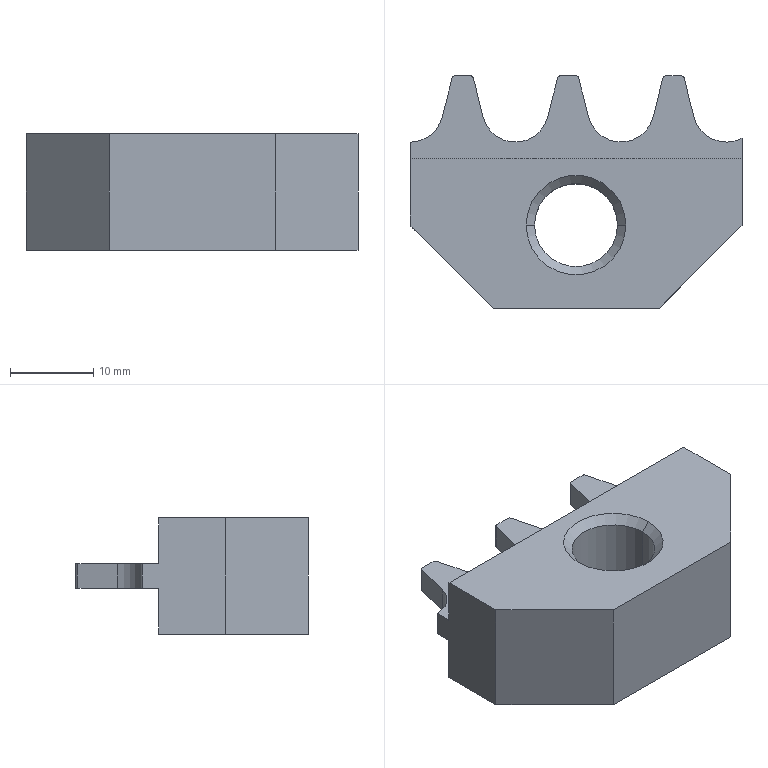Part | SolidWorks | features MirrorStock 1 | 1 solid | 36 faces | box 40 x 28 x 14 mm | volume 8141 mm3 | plane 20 | cylinder 12 | cone 4 | commonest cylinder face diameters 0.7 x6 8 x4 10 x2
STEP:
#1=CARTESIAN_POINT('',(5.,10.,-6.));
#2=VERTEX_POINT('',#1);
#3=CARTESIAN_POINT('',(-5.,10.,-6.));
#4=VERTEX_POINT('',#3);
#5=CARTESIAN_POINT('',(0.,10.,-6.));
#6=DIRECTION('',(0.,0.,1.));
#7=DIRECTION('',(-1.,0.,0.));
#8=AXIS2_PLACEMENT_3D('',#5,#6,#7);
#9=CIRCLE('',#8,5.);
#10=EDGE_CURVE('',#2,#4,#9,.T.);
#11=ORIENTED_EDGE('',*,*,#10,.T.);
#12=CARTESIAN_POINT('',(-6.,10.,-7.));
#13=VERTEX_POINT('',#12);
#14=CARTESIAN_POINT('',(-5.,10.,-6.));
#15=DIRECTION('',(-0.7071,0.,-0.7071));
#16=VECTOR('',#15,1000.);
#17=LINE('',#14,#16);
#18=EDGE_CURVE('',#4,#13,#17,.T.);
#19=ORIENTED_EDGE('',*,*,#18,.T.);
#20=CARTESIAN_POINT('',(6.,10.,-7.));
#21=VERTEX_POINT('',#20);
#22=CARTESIAN_POINT('',(0.,10.,-7.));
#23=DIRECTION('',(0.,0.,-1.));
#24=DIRECTION('',(-1.,0.,0.));
#25=AXIS2_PLACEMENT_3D('',#22,#23,#24);
#26=CIRCLE('',#25,6.);
#27=EDGE_CURVE('',#13,#21,#26,.T.);
#28=ORIENTED_EDGE('',*,*,#27,.T.);
#29=CARTESIAN_POINT('',(5.,10.,-6.));
#30=DIRECTION('',(0.7071,0.,-0.7071));
#31=VECTOR('',#30,1000.);
#32=LINE('',#29,#31);
#33=EDGE_CURVE('',#2,#21,#32,.T.);
#34=ORIENTED_EDGE('',*,*,#33,.F.);
#35=EDGE_LOOP('',(#11,#19,#28,#34));
#36=FACE_OUTER_BOUND('',#35,.T.);
#37=CARTESIAN_POINT('',(0.,10.,-6.));
#38=DIRECTION('',(0.,0.,-1.));
#39=DIRECTION('',(1.,0.,0.));
#40=AXIS2_PLACEMENT_3D('',#37,#38,#39);
#41=CONICAL_SURFACE('',#40,5.,0.7854);
#42=ADVANCED_FACE('',(#36),#41,.F.);
#43=CARTESIAN_POINT('',(-5.,10.,6.));
#44=VERTEX_POINT('',#43);
#45=CARTESIAN_POINT('',(5.,10.,6.));
#46=VERTEX_POINT('',#45);
#47=CARTESIAN_POINT('',(0.,10.,6.));
#48=DIRECTION('',(0.,0.,-1.));
#49=DIRECTION('',(-1.,0.,0.));
#50=AXIS2_PLACEMENT_3D('',#47,#48,#49);
#51=CIRCLE('',#50,5.);
#52=EDGE_CURVE('',#44,#46,#51,.T.);
#53=ORIENTED_EDGE('',*,*,#52,.T.);
#54=CARTESIAN_POINT('',(6.,10.,7.));
#55=VERTEX_POINT('',#54);
#56=CARTESIAN_POINT('',(6.,10.,7.));
#57=DIRECTION('',(0.7071,0.,0.7071));
#58=VECTOR('',#57,1000.);
#59=LINE('',#56,#58);
#60=EDGE_CURVE('',#46,#55,#59,.T.);
#61=ORIENTED_EDGE('',*,*,#60,.T.);
#62=CARTESIAN_POINT('',(-6.,10.,7.));
#63=VERTEX_POINT('',#62);
#64=CARTESIAN_POINT('',(0.,10.,7.));
#65=DIRECTION('',(0.,0.,1.));
#66=DIRECTION('',(-1.,0.,0.));
#67=AXIS2_PLACEMENT_3D('',#64,#65,#66);
#68=CIRCLE('',#67,6.);
#69=EDGE_CURVE('',#55,#63,#68,.T.);
#70=ORIENTED_EDGE('',*,*,#69,.T.);
#71=CARTESIAN_POINT('',(-6.,10.,7.));
#72=DIRECTION('',(-0.7071,0.,0.7071));
#73=VECTOR('',#72,1000.);
#74=LINE('',#71,#73);
#75=EDGE_CURVE('',#44,#63,#74,.T.);
#76=ORIENTED_EDGE('',*,*,#75,.F.);
#77=EDGE_LOOP('',(#53,#61,#70,#76));
#78=FACE_OUTER_BOUND('',#77,.T.);
#79=CARTESIAN_POINT('',(0.,10.,7.));
#80=DIRECTION('',(0.,0.,1.));
#81=DIRECTION('',(-1.,0.,0.));
#82=AXIS2_PLACEMENT_3D('',#79,#80,#81);
#83=CONICAL_SURFACE('',#82,6.,0.7854);
#84=ADVANCED_FACE('',(#78),#83,.F.);
#85=ORIENTED_EDGE('',*,*,#10,.F.);
#86=CARTESIAN_POINT('',(5.,10.,-7.));
#87=DIRECTION('',(0.,0.,1.));
#88=VECTOR('',#87,1000.);
#89=LINE('',#86,#88);
#90=EDGE_CURVE('',#2,#46,#89,.T.);
#91=ORIENTED_EDGE('',*,*,#90,.T.);
#92=ORIENTED_EDGE('',*,*,#52,.F.);
#93=CARTESIAN_POINT('',(-5.,10.,-7.));
#94=DIRECTION('',(0.,0.,1.));
#95=VECTOR('',#94,1000.);
#96=LINE('',#93,#95);
#97=EDGE_CURVE('',#4,#44,#96,.T.);
#98=ORIENTED_EDGE('',*,*,#97,.F.);
#99=EDGE_LOOP('',(#85,#91,#92,#98));
#100=FACE_OUTER_BOUND('',#99,.T.);
#101=CARTESIAN_POINT('',(0.,10.,-7.));
#102=DIRECTION('',(0.,0.,1.));
#103=DIRECTION('',(-1.,0.,0.));
#104=AXIS2_PLACEMENT_3D('',#101,#102,#103);
#105=CYLINDRICAL_SURFACE('',#104,5.);
#106=ADVANCED_FACE('',(#100),#105,.F.);
#107=CARTESIAN_POINT('',(-20.,18.,-1.5));
#108=VERTEX_POINT('',#107);
#109=CARTESIAN_POINT('',(20.,18.,-1.5));
#110=VERTEX_POINT('',#109);
#111=CARTESIAN_POINT('',(-20.,18.,-1.5));
#112=DIRECTION('',(1.,0.,0.));
#113=VECTOR('',#112,1000.);
#114=LINE('',#111,#113);
#115=EDGE_CURVE('',#108,#110,#114,.T.);
#116=ORIENTED_EDGE('',*,*,#115,.T.);
#117=CARTESIAN_POINT('',(20.,18.,-7.));
#118=VERTEX_POINT('',#117);
#119=CARTESIAN_POINT('',(20.,18.,-7.));
#120=DIRECTION('',(0.,0.,1.));
#121=VECTOR('',#120,1000.);
#122=LINE('',#119,#121);
#123=EDGE_CURVE('',#118,#110,#122,.T.);
#124=ORIENTED_EDGE('',*,*,#123,.F.);
#125=CARTESIAN_POINT('',(-20.,18.,-7.));
#126=VERTEX_POINT('',#125);
#127=CARTESIAN_POINT('',(20.,18.,-7.));
#128=DIRECTION('',(-1.,0.,0.));
#129=VECTOR('',#128,1000.);
#130=LINE('',#127,#129);
#131=EDGE_CURVE('',#118,#126,#130,.T.);
#132=ORIENTED_EDGE('',*,*,#131,.T.);
#133=CARTESIAN_POINT('',(-20.,18.,-7.));
#134=DIRECTION('',(0.,0.,1.));
#135=VECTOR('',#134,1000.);
#136=LINE('',#133,#135);
#137=EDGE_CURVE('',#126,#108,#136,.T.);
#138=ORIENTED_EDGE('',*,*,#137,.T.);
#139=EDGE_LOOP('',(#116,#124,#132,#138));
#140=FACE_OUTER_BOUND('',#139,.T.);
#141=CARTESIAN_POINT('',(20.,18.,-7.));
#142=DIRECTION('',(0.,-1.,0.));
#143=DIRECTION('',(0.,0.,1.));
#144=AXIS2_PLACEMENT_3D('',#141,#142,#143);
#145=PLANE('',#144);
#146=ADVANCED_FACE('',(#140),#145,.F.);
#147=CARTESIAN_POINT('',(0.,10.,-7.));
#148=DIRECTION('',(0.,0.,-1.));
#149=DIRECTION('',(-1.,0.,0.));
#150=AXIS2_PLACEMENT_3D('',#147,#148,#149);
#151=CIRCLE('',#150,6.);
#152=EDGE_CURVE('',#21,#13,#151,.T.);
#153=ORIENTED_EDGE('',*,*,#152,.F.);
#154=ORIENTED_EDGE('',*,*,#27,.F.);
#155=EDGE_LOOP('',(#153,#154));
#156=FACE_BOUND('',#155,.T.);
#157=CARTESIAN_POINT('',(-20.,10.,-7.));
#158=VERTEX_POINT('',#157);
#159=CARTESIAN_POINT('',(-20.,18.,-7.));
#160=DIRECTION('',(0.,-1.,0.));
#161=VECTOR('',#160,1000.);
#162=LINE('',#159,#161);
#163=EDGE_CURVE('',#126,#158,#162,.T.);
#164=ORIENTED_EDGE('',*,*,#163,.F.);
#165=ORIENTED_EDGE('',*,*,#131,.F.);
#166=CARTESIAN_POINT('',(20.,10.,-7.));
#167=VERTEX_POINT('',#166);
#168=CARTESIAN_POINT('',(20.,18.,-7.));
#169=DIRECTION('',(0.,1.,0.));
#170=VECTOR('',#169,1000.);
#171=LINE('',#168,#170);
#172=EDGE_CURVE('',#167,#118,#171,.T.);
#173=ORIENTED_EDGE('',*,*,#172,.F.);
#174=CARTESIAN_POINT('',(10.,0.,-7.));
#175=VERTEX_POINT('',#174);
#176=CARTESIAN_POINT('',(10.,0.,-7.));
#177=DIRECTION('',(0.7071,0.7071,0.));
#178=VECTOR('',#177,1000.);
#179=LINE('',#176,#178);
#180=EDGE_CURVE('',#175,#167,#179,.T.);
#181=ORIENTED_EDGE('',*,*,#180,.F.);
#182=CARTESIAN_POINT('',(-10.,0.,-7.));
#183=VERTEX_POINT('',#182);
#184=CARTESIAN_POINT('',(10.,0.,-7.));
#185=DIRECTION('',(1.,0.,0.));
#186=VECTOR('',#185,1000.);
#187=LINE('',#184,#186);
#188=EDGE_CURVE('',#183,#175,#187,.T.);
#189=ORIENTED_EDGE('',*,*,#188,.F.);
#190=CARTESIAN_POINT('',(-10.,0.,-7.));
#191=DIRECTION('',(0.7071,-0.7071,0.));
#192=VECTOR('',#191,1000.);
#193=LINE('',#190,#192);
#194=EDGE_CURVE('',#158,#183,#193,.T.);
#195=ORIENTED_EDGE('',*,*,#194,.F.);
#196=EDGE_LOOP('',(#164,#165,#173,#181,#189,#195));
#197=FACE_OUTER_BOUND('',#196,.T.);
#198=CARTESIAN_POINT('',(0.,0.,-7.));
#199=DIRECTION('',(0.,0.,1.));
#200=DIRECTION('',(-1.,0.,0.));
#201=AXIS2_PLACEMENT_3D('',#198,#199,#200);
#202=PLANE('',#201);
#203=ADVANCED_FACE('',(#156,#197),#202,.F.);
#204=CARTESIAN_POINT('',(0.,10.,7.));
#205=DIRECTION('',(0.,0.,1.));
#206=DIRECTION('',(-1.,0.,0.));
#207=AXIS2_PLACEMENT_3D('',#204,#205,#206);
#208=CIRCLE('',#207,6.);
#209=EDGE_CURVE('',#63,#55,#208,.T.);
#210=ORIENTED_EDGE('',*,*,#209,.F.);
#211=ORIENTED_EDGE('',*,*,#69,.F.);
#212=EDGE_LOOP('',(#210,#211));
#213=FACE_BOUND('',#212,.T.);
#214=CARTESIAN_POINT('',(-20.,18.,7.));
#215=VERTEX_POINT('',#214);
#216=CARTESIAN_POINT('',(-20.,10.,7.));
#217=VERTEX_POINT('',#216);
#218=CARTESIAN_POINT('',(-20.,18.,7.));
#219=DIRECTION('',(0.,-1.,0.));
#220=VECTOR('',#219,1000.);
#221=LINE('',#218,#220);
#222=EDGE_CURVE('',#215,#217,#221,.T.);
#223=ORIENTED_EDGE('',*,*,#222,.T.);
#224=CARTESIAN_POINT('',(-10.,0.,7.));
#225=VERTEX_POINT('',#224);
#226=CARTESIAN_POINT('',(-10.,0.,7.));
#227=DIRECTION('',(0.7071,-0.7071,0.));
#228=VECTOR('',#227,1000.);
#229=LINE('',#226,#228);
#230=EDGE_CURVE('',#217,#225,#229,.T.);
#231=ORIENTED_EDGE('',*,*,#230,.T.);
#232=CARTESIAN_POINT('',(10.,0.,7.));
#233=VERTEX_POINT('',#232);
#234=CARTESIAN_POINT('',(10.,0.,7.));
#235=DIRECTION('',(1.,0.,0.));
#236=VECTOR('',#235,1000.);
#237=LINE('',#234,#236);
#238=EDGE_CURVE('',#225,#233,#237,.T.);
#239=ORIENTED_EDGE('',*,*,#238,.T.);
#240=CARTESIAN_POINT('',(20.,10.,7.));
#241=VERTEX_POINT('',#240);
#242=CARTESIAN_POINT('',(10.,0.,7.));
#243=DIRECTION('',(0.7071,0.7071,0.));
#244=VECTOR('',#243,1000.);
#245=LINE('',#242,#244);
#246=EDGE_CURVE('',#233,#241,#245,.T.);
#247=ORIENTED_EDGE('',*,*,#246,.T.);
#248=CARTESIAN_POINT('',(20.,18.,7.));
#249=VERTEX_POINT('',#248);
#250=CARTESIAN_POINT('',(20.,18.,7.));
#251=DIRECTION('',(0.,1.,0.));
#252=VECTOR('',#251,1000.);
#253=LINE('',#250,#252);
#254=EDGE_CURVE('',#241,#249,#253,.T.);
#255=ORIENTED_EDGE('',*,*,#254,.T.);
#256=CARTESIAN_POINT('',(20.,18.,7.));
#257=DIRECTION('',(-1.,0.,0.));
#258=VECTOR('',#257,1000.);
#259=LINE('',#256,#258);
#260=EDGE_CURVE('',#249,#215,#259,.T.);
#261=ORIENTED_EDGE('',*,*,#260,.T.);
#262=EDGE_LOOP('',(#223,#231,#239,#247,#255,#261));
#263=FACE_OUTER_BOUND('',#262,.T.);
#264=CARTESIAN_POINT('',(0.,0.,7.));
#265=DIRECTION('',(0.,0.,1.));
#266=DIRECTION('',(-1.,0.,0.));
#267=AXIS2_PLACEMENT_3D('',#264,#265,#266);
#268=PLANE('',#267);
#269=ADVANCED_FACE('',(#213,#263),#268,.T.);
#270=ORIENTED_EDGE('',*,*,#222,.F.);
#271=CARTESIAN_POINT('',(-20.,18.,1.5));
#272=VERTEX_POINT('',#271);
#273=CARTESIAN_POINT('',(-20.,18.,-7.));
#274=DIRECTION('',(0.,0.,1.));
#275=VECTOR('',#274,1000.);
#276=LINE('',#273,#275);
#277=EDGE_CURVE('',#272,#215,#276,.T.);
#278=ORIENTED_EDGE('',*,*,#277,.F.);
#279=CARTESIAN_POINT('',(-20.,20.,1.5));
#280=VERTEX_POINT('',#279);
#281=CARTESIAN_POINT('',(-20.,18.,1.5));
#282=DIRECTION('',(0.,-1.,0.));
#283=VECTOR('',#282,1000.);
#284=LINE('',#281,#283);
#285=EDGE_CURVE('',#280,#272,#284,.T.);
#286=ORIENTED_EDGE('',*,*,#285,.F.);
#287=CARTESIAN_POINT('',(-20.,20.,-1.5));
#288=VERTEX_POINT('',#287);
#289=CARTESIAN_POINT('',(-20.,20.,-1.5));
#290=DIRECTION('',(0.,0.,1.));
#291=VECTOR('',#290,1000.);
#292=LINE('',#289,#291);
#293=EDGE_CURVE('',#288,#280,#292,.T.);
#294=ORIENTED_EDGE('',*,*,#293,.F.);
#295=CARTESIAN_POINT('',(-20.,18.,-1.5));
#296=DIRECTION('',(0.,-1.,0.));
#297=VECTOR('',#296,1000.);
#298=LINE('',#295,#297);
#299=EDGE_CURVE('',#288,#108,#298,.T.);
#300=ORIENTED_EDGE('',*,*,#299,.T.);
#301=ORIENTED_EDGE('',*,*,#137,.F.);
#302=ORIENTED_EDGE('',*,*,#163,.T.);
#303=CARTESIAN_POINT('',(-20.,10.,-7.));
#304=DIRECTION('',(0.,0.,1.));
#305=VECTOR('',#304,1000.);
#306=LINE('',#303,#305);
#307=EDGE_CURVE('',#158,#217,#306,.T.);
#308=ORIENTED_EDGE('',*,*,#307,.T.);
#309=EDGE_LOOP('',(#270,#278,#286,#294,#300,#301,#302,#308));
#310=FACE_OUTER_BOUND('',#309,.T.);
#311=CARTESIAN_POINT('',(-20.,18.,-7.));
#312=DIRECTION('',(1.,0.,0.));
#313=DIRECTION('',(0.,0.,1.));
#314=AXIS2_PLACEMENT_3D('',#311,#312,#313);
#315=PLANE('',#314);
#316=ADVANCED_FACE('',(#310),#315,.F.);
#317=ORIENTED_EDGE('',*,*,#230,.F.);
#318=ORIENTED_EDGE('',*,*,#307,.F.);
#319=ORIENTED_EDGE('',*,*,#194,.T.);
#320=CARTESIAN_POINT('',(-10.,0.,-7.));
#321=DIRECTION('',(0.,0.,1.));
#322=VECTOR('',#321,1000.);
#323=LINE('',#320,#322);
#324=EDGE_CURVE('',#183,#225,#323,.T.);
#325=ORIENTED_EDGE('',*,*,#324,.T.);
#326=EDGE_LOOP('',(#317,#318,#319,#325));
#327=FACE_OUTER_BOUND('',#326,.T.);
#328=CARTESIAN_POINT('',(-10.,0.,-7.));
#329=DIRECTION('',(0.7071,0.7071,0.));
#330=DIRECTION('',(-0.7071,0.7071,0.));
#331=AXIS2_PLACEMENT_3D('',#328,#329,#330);
#332=PLANE('',#331);
#333=ADVANCED_FACE('',(#327),#332,.F.);
#334=ORIENTED_EDGE('',*,*,#238,.F.);
#335=ORIENTED_EDGE('',*,*,#324,.F.);
#336=ORIENTED_EDGE('',*,*,#188,.T.);
#337=CARTESIAN_POINT('',(10.,0.,-7.));
#338=DIRECTION('',(0.,0.,1.));
#339=VECTOR('',#338,1000.);
#340=LINE('',#337,#339);
#341=EDGE_CURVE('',#175,#233,#340,.T.);
#342=ORIENTED_EDGE('',*,*,#341,.T.);
#343=EDGE_LOOP('',(#334,#335,#336,#342));
#344=FACE_OUTER_BOUND('',#343,.T.);
#345=CARTESIAN_POINT('',(10.,0.,-7.));
#346=DIRECTION('',(0.,1.,0.));
#347=DIRECTION('',(-1.,0.,0.));
#348=AXIS2_PLACEMENT_3D('',#345,#346,#347);
#349=PLANE('',#348);
#350=ADVANCED_FACE('',(#344),#349,.F.);
#351=ORIENTED_EDGE('',*,*,#246,.F.);
#352=ORIENTED_EDGE('',*,*,#341,.F.);
#353=ORIENTED_EDGE('',*,*,#180,.T.);
#354=CARTESIAN_POINT('',(20.,10.,-7.));
#355=DIRECTION('',(0.,0.,1.));
#356=VECTOR('',#355,1000.);
#357=LINE('',#354,#356);
#358=EDGE_CURVE('',#167,#241,#357,.T.);
#359=ORIENTED_EDGE('',*,*,#358,.T.);
#360=EDGE_LOOP('',(#351,#352,#353,#359));
#361=FACE_OUTER_BOUND('',#360,.T.);
#362=CARTESIAN_POINT('',(10.,0.,-7.));
#363=DIRECTION('',(-0.7071,0.7071,0.));
#364=DIRECTION('',(-0.7071,-0.7071,0.));
#365=AXIS2_PLACEMENT_3D('',#362,#363,#364);
#366=PLANE('',#365);
#367=ADVANCED_FACE('',(#361),#366,.F.);
#368=ORIENTED_EDGE('',*,*,#254,.F.);
#369=ORIENTED_EDGE('',*,*,#358,.F.);
#370=ORIENTED_EDGE('',*,*,#172,.T.);
#371=ORIENTED_EDGE('',*,*,#123,.T.);
#372=CARTESIAN_POINT('',(20.,20.48,-1.5));
#373=VERTEX_POINT('',#372);
#374=CARTESIAN_POINT('',(20.,18.,-1.5));
#375=DIRECTION('',(0.,1.,0.));
#376=VECTOR('',#375,1000.);
#377=LINE('',#374,#376);
#378=EDGE_CURVE('',#110,#373,#377,.T.);
#379=ORIENTED_EDGE('',*,*,#378,.T.);
#380=CARTESIAN_POINT('',(20.,20.48,1.5));
#381=VERTEX_POINT('',#380);
#382=CARTESIAN_POINT('',(20.,20.48,-1.5));
#383=DIRECTION('',(0.,0.,1.));
#384=VECTOR('',#383,1000.);
#385=LINE('',#382,#384);
#386=EDGE_CURVE('',#373,#381,#385,.T.);
#387=ORIENTED_EDGE('',*,*,#386,.T.);
#388=CARTESIAN_POINT('',(20.,18.,1.5));
#389=VERTEX_POINT('',#388);
#390=CARTESIAN_POINT('',(20.,18.,1.5));
#391=DIRECTION('',(0.,1.,0.));
#392=VECTOR('',#391,1000.);
#393=LINE('',#390,#392);
#394=EDGE_CURVE('',#389,#381,#393,.T.);
#395=ORIENTED_EDGE('',*,*,#394,.F.);
#396=CARTESIAN_POINT('',(20.,18.,-7.));
#397=DIRECTION('',(0.,0.,1.));
#398=VECTOR('',#397,1000.);
#399=LINE('',#396,#398);
#400=EDGE_CURVE('',#389,#249,#399,.T.);
#401=ORIENTED_EDGE('',*,*,#400,.T.);
#402=EDGE_LOOP('',(#368,#369,#370,#371,#379,#387,#395,#401));
#403=FACE_OUTER_BOUND('',#402,.T.);
#404=CARTESIAN_POINT('',(20.,18.,-7.));
#405=DIRECTION('',(-1.,0.,0.));
#406=DIRECTION('',(0.,0.,-1.));
#407=AXIS2_PLACEMENT_3D('',#404,#405,#406);
#408=PLANE('',#407);
#409=ADVANCED_FACE('',(#403),#408,.F.);
#410=ORIENTED_EDGE('',*,*,#277,.T.);
#411=ORIENTED_EDGE('',*,*,#260,.F.);
#412=ORIENTED_EDGE('',*,*,#400,.F.);
#413=CARTESIAN_POINT('',(-20.,18.,1.5));
#414=DIRECTION('',(1.,0.,0.));
#415=VECTOR('',#414,1000.);
#416=LINE('',#413,#415);
#417=EDGE_CURVE('',#272,#389,#416,.T.);
#418=ORIENTED_EDGE('',*,*,#417,.F.);
#419=EDGE_LOOP('',(#410,#411,#412,#418));
#420=FACE_OUTER_BOUND('',#419,.T.);
#421=CARTESIAN_POINT('',(20.,18.,-7.));
#422=DIRECTION('',(0.,-1.,0.));
#423=DIRECTION('',(0.,0.,1.));
#424=AXIS2_PLACEMENT_3D('',#421,#422,#423);
#425=PLANE('',#424);
#426=ADVANCED_FACE('',(#420),#425,.F.);
#427=ORIENTED_EDGE('',*,*,#90,.F.);
#428=CARTESIAN_POINT('',(0.,10.,-6.));
#429=DIRECTION('',(0.,0.,1.));
#430=DIRECTION('',(-1.,0.,0.));
#431=AXIS2_PLACEMENT_3D('',#428,#429,#430);
#432=CIRCLE('',#431,5.);
#433=EDGE_CURVE('',#4,#2,#432,.T.);
#434=ORIENTED_EDGE('',*,*,#433,.F.);
#435=ORIENTED_EDGE('',*,*,#97,.T.);
#436=CARTESIAN_POINT('',(0.,10.,6.));
#437=DIRECTION('',(0.,0.,-1.));
#438=DIRECTION('',(-1.,0.,0.));
#439=AXIS2_PLACEMENT_3D('',#436,#437,#438);
#440=CIRCLE('',#439,5.);
#441=EDGE_CURVE('',#46,#44,#440,.T.);
#442=ORIENTED_EDGE('',*,*,#441,.F.);
#443=EDGE_LOOP('',(#427,#434,#435,#442));
#444=FACE_OUTER_BOUND('',#443,.T.);
#445=CARTESIAN_POINT('',(0.,10.,-7.));
#446=DIRECTION('',(0.,0.,1.));
#447=DIRECTION('',(-1.,0.,0.));
#448=AXIS2_PLACEMENT_3D('',#445,#446,#447);
#449=CYLINDRICAL_SURFACE('',#448,5.);
#450=ADVANCED_FACE('',(#444),#449,.F.);
#451=CARTESIAN_POINT('',(14.224,23.01,1.5));
#452=VERTEX_POINT('',#451);
#453=CARTESIAN_POINT('',(18.1,24.,1.5));
#454=DIRECTION('',(0.,0.,-1.));
#455=DIRECTION('',(1.,0.,0.));
#456=AXIS2_PLACEMENT_3D('',#453,#454,#455);
#457=CIRCLE('',#456,4.);
#458=EDGE_CURVE('',#381,#452,#457,.T.);
#459=ORIENTED_EDGE('',*,*,#458,.F.);
#460=ORIENTED_EDGE('',*,*,#386,.F.);
#461=CARTESIAN_POINT('',(14.224,23.01,-1.5));
#462=VERTEX_POINT('',#461);
#463=CARTESIAN_POINT('',(18.1,24.,-1.5));
#464=DIRECTION('',(0.,0.,-1.));
#465=DIRECTION('',(1.,0.,0.));
#466=AXIS2_PLACEMENT_3D('',#463,#464,#465);
#467=CIRCLE('',#466,4.);
#468=EDGE_CURVE('',#373,#462,#467,.T.);
#469=ORIENTED_EDGE('',*,*,#468,.T.);
#470=CARTESIAN_POINT('',(14.224,23.01,-1.5));
#471=DIRECTION('',(0.,0.,1.));
#472=VECTOR('',#471,1000.);
#473=LINE('',#470,#472);
#474=EDGE_CURVE('',#462,#452,#473,.T.);
#475=ORIENTED_EDGE('',*,*,#474,.T.);
#476=EDGE_LOOP('',(#459,#460,#469,#475));
#477=FACE_OUTER_BOUND('',#476,.T.);
#478=CARTESIAN_POINT('',(18.1,24.,-1.5));
#479=DIRECTION('',(0.,0.,1.));
#480=DIRECTION('',(-1.,0.,0.));
#481=AXIS2_PLACEMENT_3D('',#478,#479,#480);
#482=CYLINDRICAL_SURFACE('',#481,4.);
#483=ADVANCED_FACE('',(#477),#482,.F.);
#484=CARTESIAN_POINT('',(13.017,27.737,1.5));
#485=VERTEX_POINT('',#484);
#486=CARTESIAN_POINT('',(12.95,28.,1.5));
#487=DIRECTION('',(-0.2475,0.9689,0.));
#488=VECTOR('',#487,1000.);
#489=LINE('',#486,#488);
#490=EDGE_CURVE('',#452,#485,#489,.T.);
#491=ORIENTED_EDGE('',*,*,#490,.F.);
#492=ORIENTED_EDGE('',*,*,#474,.F.);
#493=CARTESIAN_POINT('',(13.017,27.737,-1.5));
#494=VERTEX_POINT('',#493);
#495=CARTESIAN_POINT('',(12.95,28.,-1.5));
#496=DIRECTION('',(-0.2475,0.9689,0.));
#497=VECTOR('',#496,1000.);
#498=LINE('',#495,#497);
#499=EDGE_CURVE('',#462,#494,#498,.T.);
#500=ORIENTED_EDGE('',*,*,#499,.T.);
#501=CARTESIAN_POINT('',(13.017,27.737,-1.5));
#502=DIRECTION('',(0.,0.,-1.));
#503=VECTOR('',#502,1000.);
#504=LINE('',#501,#503);
#505=EDGE_CURVE('',#485,#494,#504,.T.);
#506=ORIENTED_EDGE('',*,*,#505,.F.);
#507=EDGE_LOOP('',(#491,#492,#500,#506));
#508=FACE_OUTER_BOUND('',#507,.T.);
#509=CARTESIAN_POINT('',(12.95,28.,-1.5));
#510=DIRECTION('',(-0.9689,-0.2475,0.));
#511=DIRECTION('',(0.2475,-0.9689,0.));
#512=AXIS2_PLACEMENT_3D('',#509,#510,#511);
#513=PLANE('',#512);
#514=ADVANCED_FACE('',(#508),#513,.F.);
#515=CARTESIAN_POINT('',(12.678,28.,-1.5));
#516=VERTEX_POINT('',#515);
#517=CARTESIAN_POINT('',(10.822,28.,-1.5));
#518=VERTEX_POINT('',#517);
#519=CARTESIAN_POINT('',(10.55,28.,-1.5));
#520=DIRECTION('',(-1.,0.,0.));
#521=VECTOR('',#520,1000.);
#522=LINE('',#519,#521);
#523=EDGE_CURVE('',#516,#518,#522,.T.);
#524=ORIENTED_EDGE('',*,*,#523,.T.);
#525=CARTESIAN_POINT('',(10.822,28.,1.5));
#526=VERTEX_POINT('',#525);
#527=CARTESIAN_POINT('',(10.822,28.,-1.5));
#528=DIRECTION('',(0.,0.,-1.));
#529=VECTOR('',#528,1000.);
#530=LINE('',#527,#529);
#531=EDGE_CURVE('',#526,#518,#530,.T.);
#532=ORIENTED_EDGE('',*,*,#531,.F.);
#533=CARTESIAN_POINT('',(12.678,28.,1.5));
#534=VERTEX_POINT('',#533);
#535=CARTESIAN_POINT('',(10.55,28.,1.5));
#536=DIRECTION('',(-1.,0.,0.));
#537=VECTOR('',#536,1000.);
#538=LINE('',#535,#537);
#539=EDGE_CURVE('',#534,#526,#538,.T.);
#540=ORIENTED_EDGE('',*,*,#539,.F.);
#541=CARTESIAN_POINT('',(12.678,28.,-1.5));
#542=DIRECTION('',(0.,0.,1.));
#543=VECTOR('',#542,1000.);
#544=LINE('',#541,#543);
#545=EDGE_CURVE('',#516,#534,#544,.T.);
#546=ORIENTED_EDGE('',*,*,#545,.F.);
#547=EDGE_LOOP('',(#524,#532,#540,#546));
#548=FACE_OUTER_BOUND('',#547,.T.);
#549=CARTESIAN_POINT('',(10.55,28.,-1.5));
#550=DIRECTION('',(0.,-1.,0.));
#551=DIRECTION('',(0.,0.,1.));
#552=AXIS2_PLACEMENT_3D('',#549,#550,#551);
#553=PLANE('',#552);
#554=ADVANCED_FACE('',(#548),#553,.F.);
#555=CARTESIAN_POINT('',(10.483,27.737,-1.5));
#556=VERTEX_POINT('',#555);
#557=CARTESIAN_POINT('',(9.276,23.01,-1.5));
#558=VERTEX_POINT('',#557);
#559=CARTESIAN_POINT('',(10.55,28.,-1.5));
#560=DIRECTION('',(-0.2475,-0.9689,0.));
#561=VECTOR('',#560,1000.);
#562=LINE('',#559,#561);
#563=EDGE_CURVE('',#556,#558,#562,.T.);
#564=ORIENTED_EDGE('',*,*,#563,.T.);
#565=CARTESIAN_POINT('',(9.276,23.01,1.5));
#566=VERTEX_POINT('',#565);
#567=CARTESIAN_POINT('',(9.276,23.01,-1.5));
#568=DIRECTION('',(0.,0.,1.));
#569=VECTOR('',#568,1000.);
#570=LINE('',#567,#569);
#571=EDGE_CURVE('',#558,#566,#570,.T.);
#572=ORIENTED_EDGE('',*,*,#571,.T.);
#573=CARTESIAN_POINT('',(10.483,27.737,1.5));
#574=VERTEX_POINT('',#573);
#575=CARTESIAN_POINT('',(10.55,28.,1.5));
#576=DIRECTION('',(-0.2475,-0.9689,0.));
#577=VECTOR('',#576,1000.);
#578=LINE('',#575,#577);
#579=EDGE_CURVE('',#574,#566,#578,.T.);
#580=ORIENTED_EDGE('',*,*,#579,.F.);
#581=CARTESIAN_POINT('',(10.483,27.737,-1.5));
#582=DIRECTION('',(0.,0.,1.));
#583=VECTOR('',#582,1000.);
#584=LINE('',#581,#583);
#585=EDGE_CURVE('',#556,#574,#584,.T.);
#586=ORIENTED_EDGE('',*,*,#585,.F.);
#587=EDGE_LOOP('',(#564,#572,#580,#586));
#588=FACE_OUTER_BOUND('',#587,.T.);
#589=CARTESIAN_POINT('',(10.55,28.,-1.5));
#590=DIRECTION('',(0.9689,-0.2475,0.));
#591=DIRECTION('',(0.2475,0.9689,0.));
#592=AXIS2_PLACEMENT_3D('',#589,#590,#591);
#593=PLANE('',#592);
#594=ADVANCED_FACE('',(#588),#593,.F.);
#595=CARTESIAN_POINT('',(1.524,23.01,1.5));
#596=VERTEX_POINT('',#595);
#597=CARTESIAN_POINT('',(5.4,24.,1.5));
#598=DIRECTION('',(0.,0.,-1.));
#599=DIRECTION('',(1.,0.,0.));
#600=AXIS2_PLACEMENT_3D('',#597,#598,#599);
#601=CIRCLE('',#600,4.);
#602=EDGE_CURVE('',#566,#596,#601,.T.);
#603=ORIENTED_EDGE('',*,*,#602,.F.);
#604=ORIENTED_EDGE('',*,*,#571,.F.);
#605=CARTESIAN_POINT('',(1.524,23.01,-1.5));
#606=VERTEX_POINT('',#605);
#607=CARTESIAN_POINT('',(5.4,24.,-1.5));
#608=DIRECTION('',(0.,0.,-1.));
#609=DIRECTION('',(1.,0.,0.));
#610=AXIS2_PLACEMENT_3D('',#607,#608,#609);
#611=CIRCLE('',#610,4.);
#612=EDGE_CURVE('',#558,#606,#611,.T.);
#613=ORIENTED_EDGE('',*,*,#612,.T.);
#614=CARTESIAN_POINT('',(1.524,23.01,-1.5));
#615=DIRECTION('',(0.,0.,1.));
#616=VECTOR('',#615,1000.);
#617=LINE('',#614,#616);
#618=EDGE_CURVE('',#606,#596,#617,.T.);
#619=ORIENTED_EDGE('',*,*,#618,.T.);
#620=EDGE_LOOP('',(#603,#604,#613,#619));
#621=FACE_OUTER_BOUND('',#620,.T.);
#622=CARTESIAN_POINT('',(5.4,24.,-1.5));
#623=DIRECTION('',(0.,0.,1.));
#624=DIRECTION('',(-1.,0.,0.));
#625=AXIS2_PLACEMENT_3D('',#622,#623,#624);
#626=CYLINDRICAL_SURFACE('',#625,4.);
#627=ADVANCED_FACE('',(#621),#626,.F.);
#628=CARTESIAN_POINT('',(0.3173,27.737,1.5));
#629=VERTEX_POINT('',#628);
#630=CARTESIAN_POINT('',(0.25,28.,1.5));
#631=DIRECTION('',(-0.2475,0.9689,0.));
#632=VECTOR('',#631,1000.);
#633=LINE('',#630,#632);
#634=EDGE_CURVE('',#596,#629,#633,.T.);
#635=ORIENTED_EDGE('',*,*,#634,.F.);
#636=ORIENTED_EDGE('',*,*,#618,.F.);
#637=CARTESIAN_POINT('',(0.3173,27.737,-1.5));
#638=VERTEX_POINT('',#637);
#639=CARTESIAN_POINT('',(0.25,28.,-1.5));
#640=DIRECTION('',(-0.2475,0.9689,0.));
#641=VECTOR('',#640,1000.);
#642=LINE('',#639,#641);
#643=EDGE_CURVE('',#606,#638,#642,.T.);
#644=ORIENTED_EDGE('',*,*,#643,.T.);
#645=CARTESIAN_POINT('',(0.3173,27.737,-1.5));
#646=DIRECTION('',(0.,0.,-1.));
#647=VECTOR('',#646,1000.);
#648=LINE('',#645,#647);
#649=EDGE_CURVE('',#629,#638,#648,.T.);
#650=ORIENTED_EDGE('',*,*,#649,.F.);
#651=EDGE_LOOP('',(#635,#636,#644,#650));
#652=FACE_OUTER_BOUND('',#651,.T.);
#653=CARTESIAN_POINT('',(0.25,28.,-1.5));
#654=DIRECTION('',(-0.9689,-0.2475,0.));
#655=DIRECTION('',(0.2475,-0.9689,0.));
#656=AXIS2_PLACEMENT_3D('',#653,#654,#655);
#657=PLANE('',#656);
#658=ADVANCED_FACE('',(#652),#657,.F.);
#659=CARTESIAN_POINT('',(-0.02184,28.,-1.5));
#660=VERTEX_POINT('',#659);
#661=CARTESIAN_POINT('',(-1.878,28.,-1.5));
#662=VERTEX_POINT('',#661);
#663=CARTESIAN_POINT('',(-2.15,28.,-1.5));
#664=DIRECTION('',(-1.,0.,0.));
#665=VECTOR('',#664,1000.);
#666=LINE('',#663,#665);
#667=EDGE_CURVE('',#660,#662,#666,.T.);
#668=ORIENTED_EDGE('',*,*,#667,.T.);
#669=CARTESIAN_POINT('',(-1.878,28.,1.5));
#670=VERTEX_POINT('',#669);
#671=CARTESIAN_POINT('',(-1.878,28.,-1.5));
#672=DIRECTION('',(0.,0.,-1.));
#673=VECTOR('',#672,1000.);
#674=LINE('',#671,#673);
#675=EDGE_CURVE('',#670,#662,#674,.T.);
#676=ORIENTED_EDGE('',*,*,#675,.F.);
#677=CARTESIAN_POINT('',(-0.02184,28.,1.5));
#678=VERTEX_POINT('',#677);
#679=CARTESIAN_POINT('',(-2.15,28.,1.5));
#680=DIRECTION('',(-1.,0.,0.));
#681=VECTOR('',#680,1000.);
#682=LINE('',#679,#681);
#683=EDGE_CURVE('',#678,#670,#682,.T.);
#684=ORIENTED_EDGE('',*,*,#683,.F.);
#685=CARTESIAN_POINT('',(-0.02184,28.,-1.5));
#686=DIRECTION('',(0.,0.,1.));
#687=VECTOR('',#686,1000.);
#688=LINE('',#685,#687);
#689=EDGE_CURVE('',#660,#678,#688,.T.);
#690=ORIENTED_EDGE('',*,*,#689,.F.);
#691=EDGE_LOOP('',(#668,#676,#684,#690));
#692=FACE_OUTER_BOUND('',#691,.T.);
#693=CARTESIAN_POINT('',(-2.15,28.,-1.5));
#694=DIRECTION('',(0.,-1.,0.));
#695=DIRECTION('',(0.,0.,1.));
#696=AXIS2_PLACEMENT_3D('',#693,#694,#695);
#697=PLANE('',#696);
#698=ADVANCED_FACE('',(#692),#697,.F.);
#699=CARTESIAN_POINT('',(-2.217,27.737,-1.5));
#700=VERTEX_POINT('',#699);
#701=CARTESIAN_POINT('',(-3.424,23.01,-1.5));
#702=VERTEX_POINT('',#701);
#703=CARTESIAN_POINT('',(-2.15,28.,-1.5));
#704=DIRECTION('',(-0.2475,-0.9689,0.));
#705=VECTOR('',#704,1000.);
#706=LINE('',#703,#705);
#707=EDGE_CURVE('',#700,#702,#706,.T.);
#708=ORIENTED_EDGE('',*,*,#707,.T.);
#709=CARTESIAN_POINT('',(-3.424,23.01,1.5));
#710=VERTEX_POINT('',#709);
#711=CARTESIAN_POINT('',(-3.424,23.01,-1.5));
#712=DIRECTION('',(0.,0.,1.));
#713=VECTOR('',#712,1000.);
#714=LINE('',#711,#713);
#715=EDGE_CURVE('',#702,#710,#714,.T.);
#716=ORIENTED_EDGE('',*,*,#715,.T.);
#717=CARTESIAN_POINT('',(-2.217,27.737,1.5));
#718=VERTEX_POINT('',#717);
#719=CARTESIAN_POINT('',(-2.15,28.,1.5));
#720=DIRECTION('',(-0.2475,-0.9689,0.));
#721=VECTOR('',#720,1000.);
#722=LINE('',#719,#721);
#723=EDGE_CURVE('',#718,#710,#722,.T.);
#724=ORIENTED_EDGE('',*,*,#723,.F.);
#725=CARTESIAN_POINT('',(-2.217,27.737,-1.5));
#726=DIRECTION('',(0.,0.,1.));
#727=VECTOR('',#726,1000.);
#728=LINE('',#725,#727);
#729=EDGE_CURVE('',#700,#718,#728,.T.);
#730=ORIENTED_EDGE('',*,*,#729,.F.);
#731=EDGE_LOOP('',(#708,#716,#724,#730));
#732=FACE_OUTER_BOUND('',#731,.T.);
#733=CARTESIAN_POINT('',(-2.15,28.,-1.5));
#734=DIRECTION('',(0.9689,-0.2475,0.));
#735=DIRECTION('',(0.2475,0.9689,0.));
#736=AXIS2_PLACEMENT_3D('',#733,#734,#735);
#737=PLANE('',#736);
#738=ADVANCED_FACE('',(#732),#737,.F.);
#739=CARTESIAN_POINT('',(-11.176,23.01,1.5));
#740=VERTEX_POINT('',#739);
#741=CARTESIAN_POINT('',(-7.3,24.,1.5));
#742=DIRECTION('',(0.,0.,-1.));
#743=DIRECTION('',(1.,0.,0.));
#744=AXIS2_PLACEMENT_3D('',#741,#742,#743);
#745=CIRCLE('',#744,4.);
#746=EDGE_CURVE('',#710,#740,#745,.T.);
#747=ORIENTED_EDGE('',*,*,#746,.F.);
#748=ORIENTED_EDGE('',*,*,#715,.F.);
#749=CARTESIAN_POINT('',(-11.176,23.01,-1.5));
#750=VERTEX_POINT('',#749);
#751=CARTESIAN_POINT('',(-7.3,24.,-1.5));
#752=DIRECTION('',(0.,0.,-1.));
#753=DIRECTION('',(1.,0.,0.));
#754=AXIS2_PLACEMENT_3D('',#751,#752,#753);
#755=CIRCLE('',#754,4.);
#756=EDGE_CURVE('',#702,#750,#755,.T.);
#757=ORIENTED_EDGE('',*,*,#756,.T.);
#758=CARTESIAN_POINT('',(-11.176,23.01,-1.5));
#759=DIRECTION('',(0.,0.,1.));
#760=VECTOR('',#759,1000.);
#761=LINE('',#758,#760);
#762=EDGE_CURVE('',#750,#740,#761,.T.);
#763=ORIENTED_EDGE('',*,*,#762,.T.);
#764=EDGE_LOOP('',(#747,#748,#757,#763));
#765=FACE_OUTER_BOUND('',#764,.T.);
#766=CARTESIAN_POINT('',(-7.3,24.,-1.5));
#767=DIRECTION('',(0.,0.,1.));
#768=DIRECTION('',(-1.,0.,0.));
#769=AXIS2_PLACEMENT_3D('',#766,#767,#768);
#770=CYLINDRICAL_SURFACE('',#769,4.);
#771=ADVANCED_FACE('',(#765),#770,.F.);
#772=CARTESIAN_POINT('',(-12.383,27.737,1.5));
#773=VERTEX_POINT('',#772);
#774=CARTESIAN_POINT('',(-12.45,28.,1.5));
#775=DIRECTION('',(-0.2475,0.9689,0.));
#776=VECTOR('',#775,1000.);
#777=LINE('',#774,#776);
#778=EDGE_CURVE('',#740,#773,#777,.T.);
#779=ORIENTED_EDGE('',*,*,#778,.F.);
#780=ORIENTED_EDGE('',*,*,#762,.F.);
#781=CARTESIAN_POINT('',(-12.383,27.737,-1.5));
#782=VERTEX_POINT('',#781);
#783=CARTESIAN_POINT('',(-12.45,28.,-1.5));
#784=DIRECTION('',(-0.2475,0.9689,0.));
#785=VECTOR('',#784,1000.);
#786=LINE('',#783,#785);
#787=EDGE_CURVE('',#750,#782,#786,.T.);
#788=ORIENTED_EDGE('',*,*,#787,.T.);
#789=CARTESIAN_POINT('',(-12.383,27.737,-1.5));
#790=DIRECTION('',(0.,0.,-1.));
#791=VECTOR('',#790,1000.);
#792=LINE('',#789,#791);
#793=EDGE_CURVE('',#773,#782,#792,.T.);
#794=ORIENTED_EDGE('',*,*,#793,.F.);
#795=EDGE_LOOP('',(#779,#780,#788,#794));
#796=FACE_OUTER_BOUND('',#795,.T.);
#797=CARTESIAN_POINT('',(-12.45,28.,-1.5));
#798=DIRECTION('',(-0.9689,-0.2475,0.));
#799=DIRECTION('',(0.2475,-0.9689,0.));
#800=AXIS2_PLACEMENT_3D('',#797,#798,#799);
#801=PLANE('',#800);
#802=ADVANCED_FACE('',(#796),#801,.F.);
#803=CARTESIAN_POINT('',(-12.722,28.,-1.5));
#804=VERTEX_POINT('',#803);
#805=CARTESIAN_POINT('',(-14.578,28.,-1.5));
#806=VERTEX_POINT('',#805);
#807=CARTESIAN_POINT('',(-14.85,28.,-1.5));
#808=DIRECTION('',(-1.,0.,0.));
#809=VECTOR('',#808,1000.);
#810=LINE('',#807,#809);
#811=EDGE_CURVE('',#804,#806,#810,.T.);
#812=ORIENTED_EDGE('',*,*,#811,.T.);
#813=CARTESIAN_POINT('',(-14.578,28.,1.5));
#814=VERTEX_POINT('',#813);
#815=CARTESIAN_POINT('',(-14.578,28.,-1.5));
#816=DIRECTION('',(0.,0.,-1.));
#817=VECTOR('',#816,1000.);
#818=LINE('',#815,#817);
#819=EDGE_CURVE('',#814,#806,#818,.T.);
#820=ORIENTED_EDGE('',*,*,#819,.F.);
#821=CARTESIAN_POINT('',(-12.722,28.,1.5));
#822=VERTEX_POINT('',#821);
#823=CARTESIAN_POINT('',(-14.85,28.,1.5));
#824=DIRECTION('',(-1.,0.,0.));
#825=VECTOR('',#824,1000.);
#826=LINE('',#823,#825);
#827=EDGE_CURVE('',#822,#814,#826,.T.);
#828=ORIENTED_EDGE('',*,*,#827,.F.);
#829=CARTESIAN_POINT('',(-12.722,28.,-1.5));
#830=DIRECTION('',(0.,0.,1.));
#831=VECTOR('',#830,1000.);
#832=LINE('',#829,#831);
#833=EDGE_CURVE('',#804,#822,#832,.T.);
#834=ORIENTED_EDGE('',*,*,#833,.F.);
#835=EDGE_LOOP('',(#812,#820,#828,#834));
#836=FACE_OUTER_BOUND('',#835,.T.);
#837=CARTESIAN_POINT('',(-14.85,28.,-1.5));
#838=DIRECTION('',(0.,-1.,0.));
#839=DIRECTION('',(0.,0.,1.));
#840=AXIS2_PLACEMENT_3D('',#837,#838,#839);
#841=PLANE('',#840);
#842=ADVANCED_FACE('',(#836),#841,.F.);
#843=CARTESIAN_POINT('',(-14.917,27.737,-1.5));
#844=VERTEX_POINT('',#843);
#845=CARTESIAN_POINT('',(-16.124,23.01,-1.5));
#846=VERTEX_POINT('',#845);
#847=CARTESIAN_POINT('',(-14.85,28.,-1.5));
#848=DIRECTION('',(-0.2475,-0.9689,0.));
#849=VECTOR('',#848,1000.);
#850=LINE('',#847,#849);
#851=EDGE_CURVE('',#844,#846,#850,.T.);
#852=ORIENTED_EDGE('',*,*,#851,.T.);
#853=CARTESIAN_POINT('',(-16.124,23.01,1.5));
#854=VERTEX_POINT('',#853);
#855=CARTESIAN_POINT('',(-16.124,23.01,-1.5));
#856=DIRECTION('',(0.,0.,1.));
#857=VECTOR('',#856,1000.);
#858=LINE('',#855,#857);
#859=EDGE_CURVE('',#846,#854,#858,.T.);
#860=ORIENTED_EDGE('',*,*,#859,.T.);
#861=CARTESIAN_POINT('',(-14.917,27.737,1.5));
#862=VERTEX_POINT('',#861);
#863=CARTESIAN_POINT('',(-14.85,28.,1.5));
#864=DIRECTION('',(-0.2475,-0.9689,0.));
#865=VECTOR('',#864,1000.);
#866=LINE('',#863,#865);
#867=EDGE_CURVE('',#862,#854,#866,.T.);
#868=ORIENTED_EDGE('',*,*,#867,.F.);
#869=CARTESIAN_POINT('',(-14.917,27.737,-1.5));
#870=DIRECTION('',(0.,0.,1.));
#871=VECTOR('',#870,1000.);
#872=LINE('',#869,#871);
#873=EDGE_CURVE('',#844,#862,#872,.T.);
#874=ORIENTED_EDGE('',*,*,#873,.F.);
#875=EDGE_LOOP('',(#852,#860,#868,#874));
#876=FACE_OUTER_BOUND('',#875,.T.);
#877=CARTESIAN_POINT('',(-14.85,28.,-1.5));
#878=DIRECTION('',(0.9689,-0.2475,0.));
#879=DIRECTION('',(0.2475,0.9689,0.));
#880=AXIS2_PLACEMENT_3D('',#877,#878,#879);
#881=PLANE('',#880);
#882=ADVANCED_FACE('',(#876),#881,.F.);
#883=CARTESIAN_POINT('',(-20.,24.,1.5));
#884=DIRECTION('',(0.,0.,-1.));
#885=DIRECTION('',(1.,0.,0.));
#886=AXIS2_PLACEMENT_3D('',#883,#884,#885);
#887=CIRCLE('',#886,4.);
#888=EDGE_CURVE('',#854,#280,#887,.T.);
#889=ORIENTED_EDGE('',*,*,#888,.F.);
#890=ORIENTED_EDGE('',*,*,#859,.F.);
#891=CARTESIAN_POINT('',(-20.,24.,-1.5));
#892=DIRECTION('',(0.,0.,-1.));
#893=DIRECTION('',(1.,0.,0.));
#894=AXIS2_PLACEMENT_3D('',#891,#892,#893);
#895=CIRCLE('',#894,4.);
#896=EDGE_CURVE('',#846,#288,#895,.T.);
#897=ORIENTED_EDGE('',*,*,#896,.T.);
#898=ORIENTED_EDGE('',*,*,#293,.T.);
#899=EDGE_LOOP('',(#889,#890,#897,#898));
#900=FACE_OUTER_BOUND('',#899,.T.);
#901=CARTESIAN_POINT('',(-20.,24.,-1.5));
#902=DIRECTION('',(0.,0.,1.));
#903=DIRECTION('',(-1.,0.,0.));
#904=AXIS2_PLACEMENT_3D('',#901,#902,#903);
#905=CYLINDRICAL_SURFACE('',#904,4.);
#906=ADVANCED_FACE('',(#900),#905,.F.);
#907=ORIENTED_EDGE('',*,*,#499,.F.);
#908=ORIENTED_EDGE('',*,*,#468,.F.);
#909=ORIENTED_EDGE('',*,*,#378,.F.);
#910=ORIENTED_EDGE('',*,*,#115,.F.);
#911=ORIENTED_EDGE('',*,*,#299,.F.);
#912=ORIENTED_EDGE('',*,*,#896,.F.);
#913=ORIENTED_EDGE('',*,*,#851,.F.);
#914=CARTESIAN_POINT('',(-14.578,27.65,-1.5));
#915=DIRECTION('',(0.,0.,1.));
#916=DIRECTION('',(1.,0.,0.));
#917=AXIS2_PLACEMENT_3D('',#914,#915,#916);
#918=CIRCLE('',#917,0.35);
#919=EDGE_CURVE('',#806,#844,#918,.T.);
#920=ORIENTED_EDGE('',*,*,#919,.F.);
#921=ORIENTED_EDGE('',*,*,#811,.F.);
#922=CARTESIAN_POINT('',(-12.722,27.65,-1.5));
#923=DIRECTION('',(0.,0.,1.));
#924=DIRECTION('',(1.,0.,0.));
#925=AXIS2_PLACEMENT_3D('',#922,#923,#924);
#926=CIRCLE('',#925,0.35);
#927=EDGE_CURVE('',#782,#804,#926,.T.);
#928=ORIENTED_EDGE('',*,*,#927,.F.);
#929=ORIENTED_EDGE('',*,*,#787,.F.);
#930=ORIENTED_EDGE('',*,*,#756,.F.);
#931=ORIENTED_EDGE('',*,*,#707,.F.);
#932=CARTESIAN_POINT('',(-1.878,27.65,-1.5));
#933=DIRECTION('',(0.,0.,1.));
#934=DIRECTION('',(1.,0.,0.));
#935=AXIS2_PLACEMENT_3D('',#932,#933,#934);
#936=CIRCLE('',#935,0.35);
#937=EDGE_CURVE('',#662,#700,#936,.T.);
#938=ORIENTED_EDGE('',*,*,#937,.F.);
#939=ORIENTED_EDGE('',*,*,#667,.F.);
#940=CARTESIAN_POINT('',(-0.02184,27.65,-1.5));
#941=DIRECTION('',(0.,0.,1.));
#942=DIRECTION('',(1.,0.,0.));
#943=AXIS2_PLACEMENT_3D('',#940,#941,#942);
#944=CIRCLE('',#943,0.35);
#945=EDGE_CURVE('',#638,#660,#944,.T.);
#946=ORIENTED_EDGE('',*,*,#945,.F.);
#947=ORIENTED_EDGE('',*,*,#643,.F.);
#948=ORIENTED_EDGE('',*,*,#612,.F.);
#949=ORIENTED_EDGE('',*,*,#563,.F.);
#950=CARTESIAN_POINT('',(10.822,27.65,-1.5));
#951=DIRECTION('',(0.,0.,1.));
#952=DIRECTION('',(1.,0.,0.));
#953=AXIS2_PLACEMENT_3D('',#950,#951,#952);
#954=CIRCLE('',#953,0.35);
#955=EDGE_CURVE('',#518,#556,#954,.T.);
#956=ORIENTED_EDGE('',*,*,#955,.F.);
#957=ORIENTED_EDGE('',*,*,#523,.F.);
#958=CARTESIAN_POINT('',(12.678,27.65,-1.5));
#959=DIRECTION('',(0.,0.,1.));
#960=DIRECTION('',(1.,0.,0.));
#961=AXIS2_PLACEMENT_3D('',#958,#959,#960);
#962=CIRCLE('',#961,0.35);
#963=EDGE_CURVE('',#494,#516,#962,.T.);
#964=ORIENTED_EDGE('',*,*,#963,.F.);
#965=EDGE_LOOP('',(#907,#908,#909,#910,#911,#912,#913,#920,#921,#928,#929,#930,#931,#938,#939,#946,#947,#948,#949,#956,#957,#964));
#966=FACE_OUTER_BOUND('',#965,.T.);
#967=CARTESIAN_POINT('',(18.1,24.,-1.5));
#968=DIRECTION('',(0.,0.,-1.));
#969=DIRECTION('',(1.,0.,0.));
#970=AXIS2_PLACEMENT_3D('',#967,#968,#969);
#971=PLANE('',#970);
#972=ADVANCED_FACE('',(#966),#971,.T.);
#973=ORIENTED_EDGE('',*,*,#539,.T.);
#974=CARTESIAN_POINT('',(10.822,27.65,1.5));
#975=DIRECTION('',(0.,0.,-1.));
#976=DIRECTION('',(1.,0.,0.));
#977=AXIS2_PLACEMENT_3D('',#974,#975,#976);
#978=CIRCLE('',#977,0.35);
#979=EDGE_CURVE('',#574,#526,#978,.T.);
#980=ORIENTED_EDGE('',*,*,#979,.F.);
#981=ORIENTED_EDGE('',*,*,#579,.T.);
#982=ORIENTED_EDGE('',*,*,#602,.T.);
#983=ORIENTED_EDGE('',*,*,#634,.T.);
#984=CARTESIAN_POINT('',(-0.02184,27.65,1.5));
#985=DIRECTION('',(0.,0.,-1.));
#986=DIRECTION('',(1.,0.,0.));
#987=AXIS2_PLACEMENT_3D('',#984,#985,#986);
#988=CIRCLE('',#987,0.35);
#989=EDGE_CURVE('',#678,#629,#988,.T.);
#990=ORIENTED_EDGE('',*,*,#989,.F.);
#991=ORIENTED_EDGE('',*,*,#683,.T.);
#992=CARTESIAN_POINT('',(-1.878,27.65,1.5));
#993=DIRECTION('',(0.,0.,-1.));
#994=DIRECTION('',(1.,0.,0.));
#995=AXIS2_PLACEMENT_3D('',#992,#993,#994);
#996=CIRCLE('',#995,0.35);
#997=EDGE_CURVE('',#718,#670,#996,.T.);
#998=ORIENTED_EDGE('',*,*,#997,.F.);
#999=ORIENTED_EDGE('',*,*,#723,.T.);
#1000=ORIENTED_EDGE('',*,*,#746,.T.);
#1001=ORIENTED_EDGE('',*,*,#778,.T.);
#1002=CARTESIAN_POINT('',(-12.722,27.65,1.5));
#1003=DIRECTION('',(0.,0.,-1.));
#1004=DIRECTION('',(1.,0.,0.));
#1005=AXIS2_PLACEMENT_3D('',#1002,#1003,#1004);
#1006=CIRCLE('',#1005,0.35);
#1007=EDGE_CURVE('',#822,#773,#1006,.T.);
#1008=ORIENTED_EDGE('',*,*,#1007,.F.);
#1009=ORIENTED_EDGE('',*,*,#827,.T.);
#1010=CARTESIAN_POINT('',(-14.578,27.65,1.5));
#1011=DIRECTION('',(0.,0.,-1.));
#1012=DIRECTION('',(1.,0.,0.));
#1013=AXIS2_PLACEMENT_3D('',#1010,#1011,#1012);
#1014=CIRCLE('',#1013,0.35);
#1015=EDGE_CURVE('',#862,#814,#1014,.T.);
#1016=ORIENTED_EDGE('',*,*,#1015,.F.);
#1017=ORIENTED_EDGE('',*,*,#867,.T.);
#1018=ORIENTED_EDGE('',*,*,#888,.T.);
#1019=ORIENTED_EDGE('',*,*,#285,.T.);
#1020=ORIENTED_EDGE('',*,*,#417,.T.);
#1021=ORIENTED_EDGE('',*,*,#394,.T.);
#1022=ORIENTED_EDGE('',*,*,#458,.T.);
#1023=ORIENTED_EDGE('',*,*,#490,.T.);
#1024=CARTESIAN_POINT('',(12.678,27.65,1.5));
#1025=DIRECTION('',(0.,0.,-1.));
#1026=DIRECTION('',(1.,0.,0.));
#1027=AXIS2_PLACEMENT_3D('',#1024,#1025,#1026);
#1028=CIRCLE('',#1027,0.35);
#1029=EDGE_CURVE('',#534,#485,#1028,.T.);
#1030=ORIENTED_EDGE('',*,*,#1029,.F.);
#1031=EDGE_LOOP('',(#973,#980,#981,#982,#983,#990,#991,#998,#999,#1000,#1001,#1008,#1009,#1016,#1017,#1018,#1019,#1020,#1021,#1022,#1023,#1030));
#1032=FACE_OUTER_BOUND('',#1031,.T.);
#1033=CARTESIAN_POINT('',(18.1,24.,1.5));
#1034=DIRECTION('',(0.,0.,-1.));
#1035=DIRECTION('',(1.,0.,0.));
#1036=AXIS2_PLACEMENT_3D('',#1033,#1034,#1035);
#1037=PLANE('',#1036);
#1038=ADVANCED_FACE('',(#1032),#1037,.F.);
#1039=ORIENTED_EDGE('',*,*,#963,.T.);
#1040=ORIENTED_EDGE('',*,*,#545,.T.);
#1041=ORIENTED_EDGE('',*,*,#1029,.T.);
#1042=ORIENTED_EDGE('',*,*,#505,.T.);
#1043=EDGE_LOOP('',(#1039,#1040,#1041,#1042));
#1044=FACE_OUTER_BOUND('',#1043,.T.);
#1045=CARTESIAN_POINT('',(12.678,27.65,-1.5));
#1046=DIRECTION('',(0.,0.,1.));
#1047=DIRECTION('',(-1.,0.,0.));
#1048=AXIS2_PLACEMENT_3D('',#1045,#1046,#1047);
#1049=CYLINDRICAL_SURFACE('',#1048,0.35);
#1050=ADVANCED_FACE('',(#1044),#1049,.T.);
#1051=ORIENTED_EDGE('',*,*,#955,.T.);
#1052=ORIENTED_EDGE('',*,*,#585,.T.);
#1053=ORIENTED_EDGE('',*,*,#979,.T.);
#1054=ORIENTED_EDGE('',*,*,#531,.T.);
#1055=EDGE_LOOP('',(#1051,#1052,#1053,#1054));
#1056=FACE_OUTER_BOUND('',#1055,.T.);
#1057=CARTESIAN_POINT('',(10.822,27.65,-1.5));
#1058=DIRECTION('',(0.,0.,1.));
#1059=DIRECTION('',(-1.,0.,0.));
#1060=AXIS2_PLACEMENT_3D('',#1057,#1058,#1059);
#1061=CYLINDRICAL_SURFACE('',#1060,0.35);
#1062=ADVANCED_FACE('',(#1056),#1061,.T.);
#1063=ORIENTED_EDGE('',*,*,#945,.T.);
#1064=ORIENTED_EDGE('',*,*,#689,.T.);
#1065=ORIENTED_EDGE('',*,*,#989,.T.);
#1066=ORIENTED_EDGE('',*,*,#649,.T.);
#1067=EDGE_LOOP('',(#1063,#1064,#1065,#1066));
#1068=FACE_OUTER_BOUND('',#1067,.T.);
#1069=CARTESIAN_POINT('',(-0.02184,27.65,-1.5));
#1070=DIRECTION('',(0.,0.,1.));
#1071=DIRECTION('',(-1.,0.,0.));
#1072=AXIS2_PLACEMENT_3D('',#1069,#1070,#1071);
#1073=CYLINDRICAL_SURFACE('',#1072,0.35);
#1074=ADVANCED_FACE('',(#1068),#1073,.T.);
#1075=ORIENTED_EDGE('',*,*,#937,.T.);
#1076=ORIENTED_EDGE('',*,*,#729,.T.);
#1077=ORIENTED_EDGE('',*,*,#997,.T.);
#1078=ORIENTED_EDGE('',*,*,#675,.T.);
#1079=EDGE_LOOP('',(#1075,#1076,#1077,#1078));
#1080=FACE_OUTER_BOUND('',#1079,.T.);
#1081=CARTESIAN_POINT('',(-1.878,27.65,-1.5));
#1082=DIRECTION('',(0.,0.,1.));
#1083=DIRECTION('',(-1.,0.,0.));
#1084=AXIS2_PLACEMENT_3D('',#1081,#1082,#1083);
#1085=CYLINDRICAL_SURFACE('',#1084,0.35);
#1086=ADVANCED_FACE('',(#1080),#1085,.T.);
#1087=ORIENTED_EDGE('',*,*,#927,.T.);
#1088=ORIENTED_EDGE('',*,*,#833,.T.);
#1089=ORIENTED_EDGE('',*,*,#1007,.T.);
#1090=ORIENTED_EDGE('',*,*,#793,.T.);
#1091=EDGE_LOOP('',(#1087,#1088,#1089,#1090));
#1092=FACE_OUTER_BOUND('',#1091,.T.);
#1093=CARTESIAN_POINT('',(-12.722,27.65,-1.5));
#1094=DIRECTION('',(0.,0.,1.));
#1095=DIRECTION('',(-1.,0.,0.));
#1096=AXIS2_PLACEMENT_3D('',#1093,#1094,#1095);
#1097=CYLINDRICAL_SURFACE('',#1096,0.35);
#1098=ADVANCED_FACE('',(#1092),#1097,.T.);
#1099=ORIENTED_EDGE('',*,*,#919,.T.);
#1100=ORIENTED_EDGE('',*,*,#873,.T.);
#1101=ORIENTED_EDGE('',*,*,#1015,.T.);
#1102=ORIENTED_EDGE('',*,*,#819,.T.);
#1103=EDGE_LOOP('',(#1099,#1100,#1101,#1102));
#1104=FACE_OUTER_BOUND('',#1103,.T.);
#1105=CARTESIAN_POINT('',(-14.578,27.65,-1.5));
#1106=DIRECTION('',(0.,0.,1.));
#1107=DIRECTION('',(-1.,0.,0.));
#1108=AXIS2_PLACEMENT_3D('',#1105,#1106,#1107);
#1109=CYLINDRICAL_SURFACE('',#1108,0.35);
#1110=ADVANCED_FACE('',(#1104),#1109,.T.);
#1111=ORIENTED_EDGE('',*,*,#60,.F.);
#1112=ORIENTED_EDGE('',*,*,#441,.T.);
#1113=ORIENTED_EDGE('',*,*,#75,.T.);
#1114=ORIENTED_EDGE('',*,*,#209,.T.);
#1115=EDGE_LOOP('',(#1111,#1112,#1113,#1114));
#1116=FACE_OUTER_BOUND('',#1115,.T.);
#1117=CARTESIAN_POINT('',(0.,10.,7.));
#1118=DIRECTION('',(0.,0.,1.));
#1119=DIRECTION('',(-1.,0.,0.));
#1120=AXIS2_PLACEMENT_3D('',#1117,#1118,#1119);
#1121=CONICAL_SURFACE('',#1120,6.,0.7854);
#1122=ADVANCED_FACE('',(#1116),#1121,.F.);
#1123=ORIENTED_EDGE('',*,*,#18,.F.);
#1124=ORIENTED_EDGE('',*,*,#433,.T.);
#1125=ORIENTED_EDGE('',*,*,#33,.T.);
#1126=ORIENTED_EDGE('',*,*,#152,.T.);
#1127=EDGE_LOOP('',(#1123,#1124,#1125,#1126));
#1128=FACE_OUTER_BOUND('',#1127,.T.);
#1129=CARTESIAN_POINT('',(0.,10.,-6.));
#1130=DIRECTION('',(0.,0.,-1.));
#1131=DIRECTION('',(1.,0.,0.));
#1132=AXIS2_PLACEMENT_3D('',#1129,#1130,#1131);
#1133=CONICAL_SURFACE('',#1132,5.,0.7854);
#1134=ADVANCED_FACE('',(#1128),#1133,.F.);
#1135=CLOSED_SHELL('',(#42,#84,#106,#146,#203,#269,#316,#333,#350,#367,#409,#426,#450,#483,#514,#554,#594,#627,#658,#698,#738,#771,#802,#842,#882,#906,#972,#1038,#1050,#1062,#1074,#1086,#1098,#1110,#1122,#1134));
#1136=MANIFOLD_SOLID_BREP('',#1135);
#1137=CARTESIAN_POINT('',(0.,0.,0.));
#1138=DIRECTION('',(0.,0.,1.));
#1139=DIRECTION('',(1.,0.,0.));
#1140=AXIS2_PLACEMENT_3D('',#1137,#1138,#1139);
#1141=(LENGTH_UNIT()NAMED_UNIT(*)SI_UNIT(.MILLI.,.METRE.));
#1142=UNCERTAINTY_MEASURE_WITH_UNIT(LENGTH_MEASURE(0.00001),#1141,'','');
#1143=(NAMED_UNIT(*)PLANE_ANGLE_UNIT()SI_UNIT($,.RADIAN.));
#1144=(NAMED_UNIT(*)SI_UNIT($,.STERADIAN.)SOLID_ANGLE_UNIT());
#1145=(GEOMETRIC_REPRESENTATION_CONTEXT(3)GLOBAL_UNCERTAINTY_ASSIGNED_CONTEXT((#1142))GLOBAL_UNIT_ASSIGNED_CONTEXT((#1141,#1143,#1144))REPRESENTATION_CONTEXT('',''));
#1146=ADVANCED_BREP_SHAPE_REPRESENTATION('',(#1136,#1140),#1145);